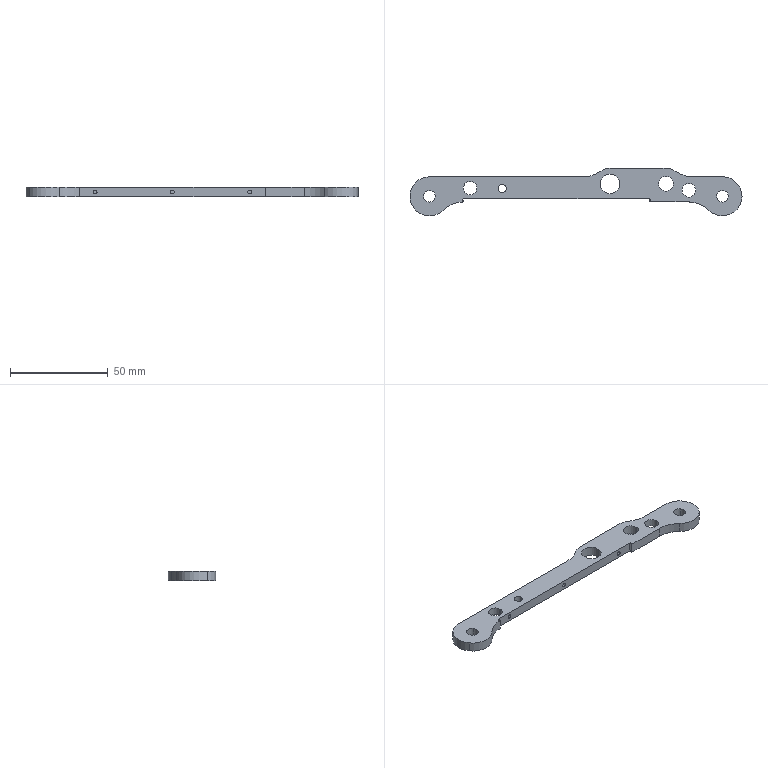Part | NX | features BREP 1 | 1 solid | 52 faces | box 170 x 24.378 x 5 mm | volume 10473 mm3 | cylinder 37 | plane 15 | commonest cylinder face diameters 2 x6 10 x6 6 x4 7 x4 30 x4 1 x3